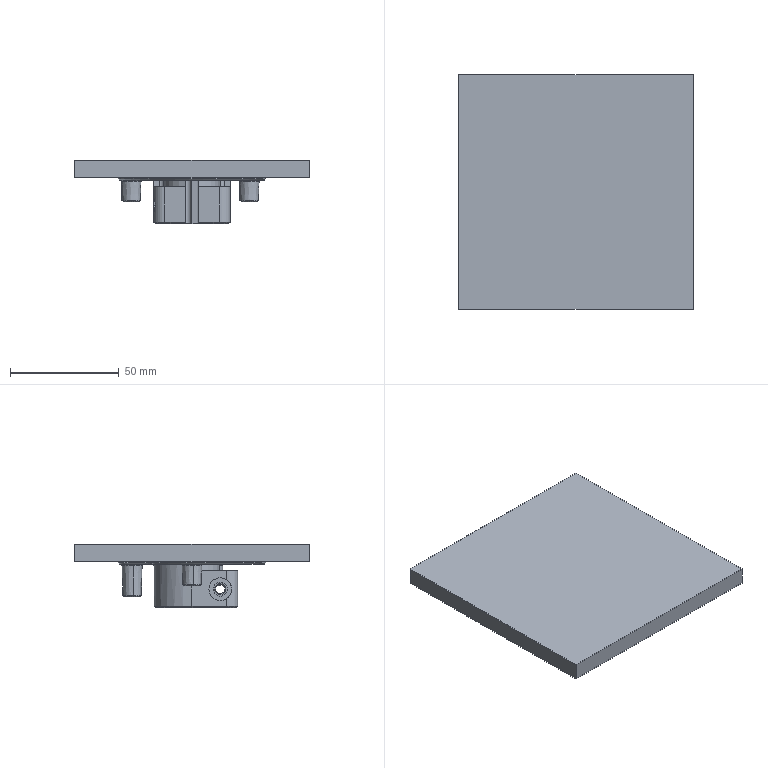NC program | NX | posted with a generic post | part box 108 x 108 x 29 mm
Lines 1 to 66 of 13118:
N10 G17 G21 G94 G90
(FLOOR_WALL_COPY , TOOL : D63)
N12 T03 M6
N14 G54
N16 G17 G0 G90 X-68.499 Y33.998 S6500 M3
N18 G43 Z30. H3
N20 Z3.
N22 G94 G1 Z0. F1250.
N24 X-65.499
N26 X65.499
N28 Y-8.799
N30 X-65.499
N32 X-68.499
N34 Z3.
N36 G0 Z30.
N38 M5
(DRILLING_COPY_1 , TOOL : D6A45)
N40 T01 M6
N42 G54
N44 G17 G0 G90 X-28. Y0. S5000 M3
N46 G43 Z30. H1
N48 G94 G81 G98 Z-1. F250. R3.
N50 X0.
N52 X-1.997 Y11.325
N54 X4.862 Y27.575
N56 X26.311 Y-9.577
N58 G80
N60 G0 X26.311 Y-9.577 Z30.
N62 M5
(DRILLING_COPY_1_COPY , TOOL : 5.1ZT)
N64 T11 M6
N66 G54
N68 G17 G0 G90 X4.862 Y27.575 S2000 M3
N70 G43 Z30. H11
N72 G94 G83 G98 Z-23.032 F250. Q2. R3.
N74 X26.311 Y-9.577 Z-18.032
N76 X-28. Y0.
N78 G80
N80 G0 X-28. Y0. Z30.
(DRILLING_COPY_1_COPY_COPY_1 , TOOL : 5.1ZT)
N82 X0.
N84 G83 Z-28.032 F250. Q2. R3.
N86 G80
N88 G0 X0. Y0. Z30.
N90 M5
(DRILLING_COPY_1_COPY_COPY , TOOL : 3.0ZT)
N92 T12 M6
N94 G54
N96 G17 G0 G90 X-1.997 Y11.325 S2122 M3
N98 G43 Z30. H12
N100 G94 G83 G98 Z-27.401 F150. Q2. R3.
N102 G80
N104 G0 X-1.997 Y11.325 Z30.
N106 M5